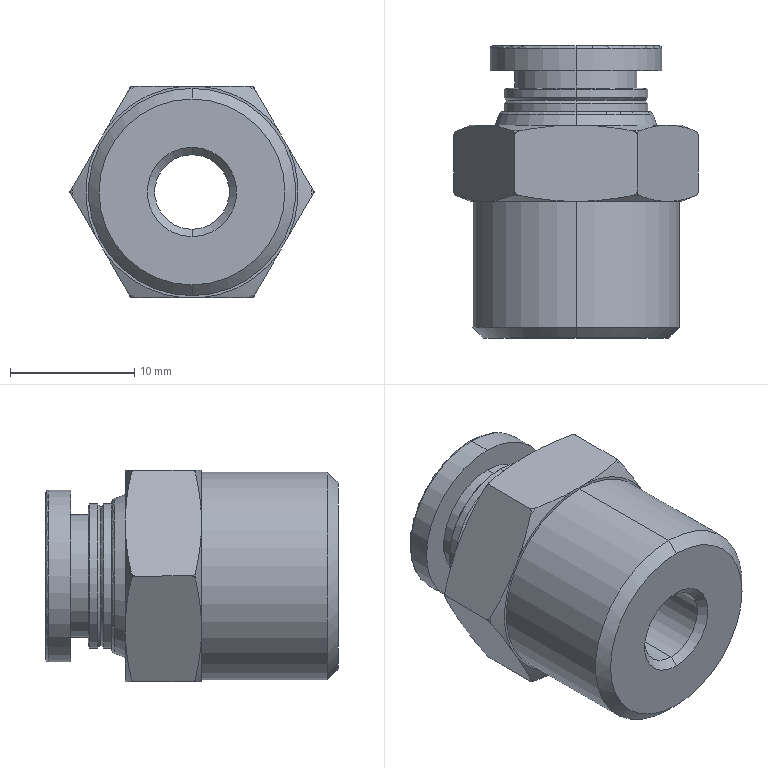Part | NX | features BREP 1 | 1 solid | 70 faces | box 19.63 x 23.5 x 17 mm | volume 3569 mm3 | cone 24 | torus 18 | cylinder 14 | plane 14 | commonest cylinder face diameters 11.6 x4 6 x2 8 x2 9.9 x2 13.8 x2 16.662 x2